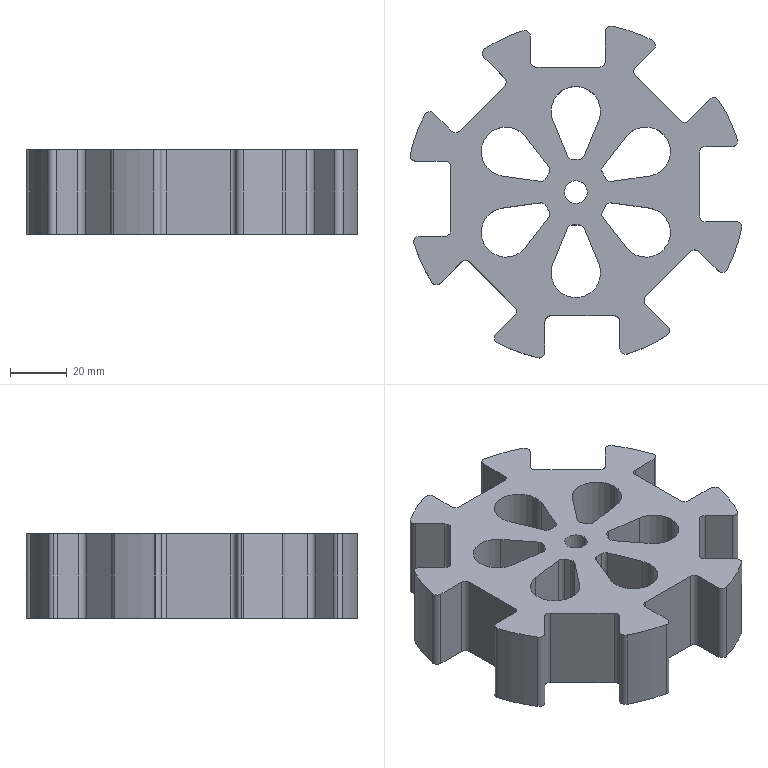Part | SolidWorks | features ICE 2, CirPattern 1, Extrusion 1, Fillet 1 | 1 solid | 121 faces | box 117.193 x 117.193 x 30 mm | volume 181136 mm3 | cylinder 76 | plane 45 | commonest cylinder face diameters 4 x52 17.43 x12 120 x8 1.367 x2 8 x2